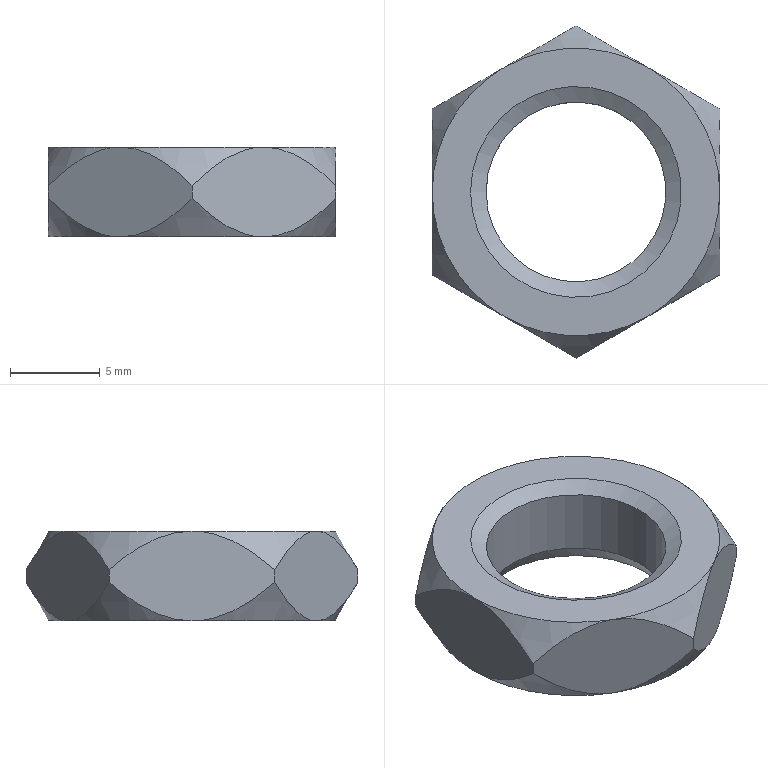Part | NX | features solid 2 | 1 solid | 23 faces | box 16 x 18.475 x 5 mm | volume 674.901 mm3 | cone 14 | plane 8 | cylinder 1 | commonest cylinder face diameters 10 x1
STEP:
#1=CARTESIAN_POINT('',(-5.5,537.,-71.));
#2=VERTEX_POINT('',#1);
#3=CARTESIAN_POINT('',(0.,537.,-71.));
#4=DIRECTION('',(0.,0.,-1.));
#5=DIRECTION('',(-1.,0.,0.));
#6=AXIS2_PLACEMENT_3D('',#3,#4,#5);
#7=CIRCLE('',#6,5.5);
#8=EDGE_CURVE('',#2,#2,#7,.F.);
#9=ORIENTED_EDGE('',*,*,#8,.T.);
#10=EDGE_LOOP('',(#9));
#11=FACE_BOUND('',#10,.T.);
#12=CARTESIAN_POINT('',(-8.,537.,-71.));
#13=VERTEX_POINT('',#12);
#14=CARTESIAN_POINT('',(-4.,530.072,-71.));
#15=VERTEX_POINT('',#14);
#16=CARTESIAN_POINT('',(0.,537.,-71.));
#17=DIRECTION('',(0.,0.,1.));
#18=DIRECTION('',(1.,0.,0.));
#19=AXIS2_PLACEMENT_3D('',#16,#17,#18);
#20=CIRCLE('',#19,8.);
#21=EDGE_CURVE('',#13,#15,#20,.T.);
#22=ORIENTED_EDGE('',*,*,#21,.F.);
#23=CARTESIAN_POINT('',(-4.,543.928,-71.));
#24=VERTEX_POINT('',#23);
#25=CARTESIAN_POINT('',(0.,537.,-71.));
#26=DIRECTION('',(0.,0.,1.));
#27=DIRECTION('',(1.,0.,0.));
#28=AXIS2_PLACEMENT_3D('',#25,#26,#27);
#29=CIRCLE('',#28,8.);
#30=EDGE_CURVE('',#24,#13,#29,.T.);
#31=ORIENTED_EDGE('',*,*,#30,.F.);
#32=CARTESIAN_POINT('',(4.,543.928,-71.));
#33=VERTEX_POINT('',#32);
#34=CARTESIAN_POINT('',(0.,537.,-71.));
#35=DIRECTION('',(0.,0.,1.));
#36=DIRECTION('',(1.,0.,0.));
#37=AXIS2_PLACEMENT_3D('',#34,#35,#36);
#38=CIRCLE('',#37,8.);
#39=EDGE_CURVE('',#33,#24,#38,.T.);
#40=ORIENTED_EDGE('',*,*,#39,.F.);
#41=CARTESIAN_POINT('',(8.,537.,-71.));
#42=VERTEX_POINT('',#41);
#43=CARTESIAN_POINT('',(0.,537.,-71.));
#44=DIRECTION('',(0.,0.,1.));
#45=DIRECTION('',(1.,0.,0.));
#46=AXIS2_PLACEMENT_3D('',#43,#44,#45);
#47=CIRCLE('',#46,8.);
#48=EDGE_CURVE('',#42,#33,#47,.T.);
#49=ORIENTED_EDGE('',*,*,#48,.F.);
#50=CARTESIAN_POINT('',(4.,530.072,-71.));
#51=VERTEX_POINT('',#50);
#52=CARTESIAN_POINT('',(0.,537.,-71.));
#53=DIRECTION('',(0.,0.,1.));
#54=DIRECTION('',(1.,0.,0.));
#55=AXIS2_PLACEMENT_3D('',#52,#53,#54);
#56=CIRCLE('',#55,8.);
#57=EDGE_CURVE('',#51,#42,#56,.T.);
#58=ORIENTED_EDGE('',*,*,#57,.F.);
#59=CARTESIAN_POINT('',(0.,537.,-71.));
#60=DIRECTION('',(0.,0.,1.));
#61=DIRECTION('',(1.,0.,0.));
#62=AXIS2_PLACEMENT_3D('',#59,#60,#61);
#63=CIRCLE('',#62,8.);
#64=EDGE_CURVE('',#15,#51,#63,.T.);
#65=ORIENTED_EDGE('',*,*,#64,.F.);
#66=EDGE_LOOP('',(#22,#31,#40,#49,#58,#65));
#67=FACE_BOUND('',#66,.T.);
#68=CARTESIAN_POINT('',(-16.,537.,-71.));
#69=DIRECTION('',(0.,0.,-1.));
#70=DIRECTION('',(-1.,0.,0.));
#71=AXIS2_PLACEMENT_3D('',#68,#69,#70);
#72=PLANE('',#71);
#73=ADVANCED_FACE('',(#11,#67),#72,.T.);
#74=CARTESIAN_POINT('',(-8.,532.381,-68.144));
#75=VERTEX_POINT('',#74);
#76=CARTESIAN_POINT('',(-4.,530.072,-66.));
#77=VERTEX_POINT('',#76);
#78=CARTESIAN_POINT('',(-8.,532.381,-68.144));
#79=CARTESIAN_POINT('',(-7.431,532.053,-67.575));
#80=CARTESIAN_POINT('',(-6.238,531.364,-66.534));
#81=CARTESIAN_POINT('',(-4.752,530.506,-66.));
#82=CARTESIAN_POINT('',(-4.,530.072,-66.));
#83=B_SPLINE_CURVE_WITH_KNOTS('',3,(#78,#79,#80,#81,#82),.UNSPECIFIED.,.F.,.F.,(4,1,4),(0.000000303,0.002586,0.005171),.UNSPECIFIED.);
#84=EDGE_CURVE('',#75,#77,#83,.T.);
#85=ORIENTED_EDGE('',*,*,#84,.F.);
#86=CARTESIAN_POINT('',(-8.,532.381,-68.856));
#87=VERTEX_POINT('',#86);
#88=CARTESIAN_POINT('',(-8.,532.381,-66.));
#89=DIRECTION('',(0.,0.,-1.));
#90=VECTOR('',#89,1000.);
#91=LINE('',#88,#90);
#92=EDGE_CURVE('',#75,#87,#91,.T.);
#93=ORIENTED_EDGE('',*,*,#92,.T.);
#94=CARTESIAN_POINT('',(-8.,532.381,-68.856));
#95=CARTESIAN_POINT('',(-7.431,532.053,-69.425));
#96=CARTESIAN_POINT('',(-6.238,531.364,-70.466));
#97=CARTESIAN_POINT('',(-4.752,530.506,-71.));
#98=CARTESIAN_POINT('',(-4.,530.072,-71.));
#99=B_SPLINE_CURVE_WITH_KNOTS('',3,(#94,#95,#96,#97,#98),.UNSPECIFIED.,.F.,.F.,(4,1,4),(0.000000303,0.002586,0.005171),.UNSPECIFIED.);
#100=EDGE_CURVE('',#87,#15,#99,.T.);
#101=ORIENTED_EDGE('',*,*,#100,.T.);
#102=CARTESIAN_POINT('',(0.,527.762,-68.856));
#103=VERTEX_POINT('',#102);
#104=CARTESIAN_POINT('',(-4.,530.072,-71.));
#105=CARTESIAN_POINT('',(-2.498,529.205,-71.));
#106=CARTESIAN_POINT('',(-1.14,528.42,-69.996));
#107=CARTESIAN_POINT('',(0.,527.762,-68.856));
#108=B_SPLINE_CURVE_WITH_KNOTS('',3,(#104,#105,#106,#107),.UNSPECIFIED.,.F.,.F.,(4,4),(0.005171,0.01033),.UNSPECIFIED.);
#109=EDGE_CURVE('',#15,#103,#108,.T.);
#110=ORIENTED_EDGE('',*,*,#109,.T.);
#111=CARTESIAN_POINT('',(0.,527.762,-68.144));
#112=VERTEX_POINT('',#111);
#113=CARTESIAN_POINT('',(0.,527.762,-66.));
#114=DIRECTION('',(0.,0.,-1.));
#115=VECTOR('',#114,1000.);
#116=LINE('',#113,#115);
#117=EDGE_CURVE('',#112,#103,#116,.T.);
#118=ORIENTED_EDGE('',*,*,#117,.F.);
#119=CARTESIAN_POINT('',(-4.,530.072,-66.));
#120=CARTESIAN_POINT('',(-2.498,529.205,-66.));
#121=CARTESIAN_POINT('',(-1.14,528.42,-67.004));
#122=CARTESIAN_POINT('',(0.,527.762,-68.144));
#123=B_SPLINE_CURVE_WITH_KNOTS('',3,(#119,#120,#121,#122),.UNSPECIFIED.,.F.,.F.,(4,4),(0.005171,0.01033),.UNSPECIFIED.);
#124=EDGE_CURVE('',#77,#112,#123,.T.);
#125=ORIENTED_EDGE('',*,*,#124,.F.);
#126=EDGE_LOOP('',(#85,#93,#101,#110,#118,#125));
#127=FACE_BOUND('',#126,.T.);
#128=CARTESIAN_POINT('',(0.,527.762,-66.));
#129=DIRECTION('',(-0.5,-0.866,0.));
#130=DIRECTION('',(0.866,-0.5,0.));
#131=AXIS2_PLACEMENT_3D('',#128,#129,#130);
#132=PLANE('',#131);
#133=ADVANCED_FACE('',(#127),#132,.T.);
#134=CARTESIAN_POINT('',(-8.,541.619,-68.144));
#135=VERTEX_POINT('',#134);
#136=CARTESIAN_POINT('',(-8.,537.,-66.));
#137=VERTEX_POINT('',#136);
#138=CARTESIAN_POINT('',(-8.,537.,-66.));
#139=CARTESIAN_POINT('',(-8.,538.745,-66.));
#140=CARTESIAN_POINT('',(-8.,540.316,-67.015));
#141=CARTESIAN_POINT('',(-8.,541.619,-68.144));
#142=B_SPLINE_CURVE_WITH_KNOTS('',3,(#138,#139,#140,#141),.UNSPECIFIED.,.F.,.F.,(4,4),(0.01058,0.01572),.UNSPECIFIED.);
#143=EDGE_CURVE('',#135,#137,#142,.F.);
#144=ORIENTED_EDGE('',*,*,#143,.F.);
#145=CARTESIAN_POINT('',(-8.,541.619,-68.856));
#146=VERTEX_POINT('',#145);
#147=CARTESIAN_POINT('',(-8.,541.619,-66.));
#148=DIRECTION('',(0.,0.,-1.));
#149=VECTOR('',#148,1000.);
#150=LINE('',#147,#149);
#151=EDGE_CURVE('',#135,#146,#150,.T.);
#152=ORIENTED_EDGE('',*,*,#151,.T.);
#153=CARTESIAN_POINT('',(-8.,537.,-71.));
#154=CARTESIAN_POINT('',(-8.,538.745,-71.));
#155=CARTESIAN_POINT('',(-8.,540.316,-69.985));
#156=CARTESIAN_POINT('',(-8.,541.619,-68.856));
#157=B_SPLINE_CURVE_WITH_KNOTS('',3,(#153,#154,#155,#156),.UNSPECIFIED.,.F.,.F.,(4,4),(0.01058,0.01572),.UNSPECIFIED.);
#158=EDGE_CURVE('',#146,#13,#157,.F.);
#159=ORIENTED_EDGE('',*,*,#158,.T.);
#160=CARTESIAN_POINT('',(-8.,532.381,-68.856));
#161=CARTESIAN_POINT('',(-8.,533.681,-69.982));
#162=CARTESIAN_POINT('',(-8.,535.253,-71.));
#163=CARTESIAN_POINT('',(-8.,537.,-71.));
#164=B_SPLINE_CURVE_WITH_KNOTS('',3,(#160,#161,#162,#163),.UNSPECIFIED.,.F.,.F.,(4,4),(0.005438,0.01058),.UNSPECIFIED.);
#165=EDGE_CURVE('',#13,#87,#164,.F.);
#166=ORIENTED_EDGE('',*,*,#165,.T.);
#167=ORIENTED_EDGE('',*,*,#92,.F.);
#168=CARTESIAN_POINT('',(-8.,532.381,-68.144));
#169=CARTESIAN_POINT('',(-8.,533.681,-67.018));
#170=CARTESIAN_POINT('',(-8.,535.253,-66.));
#171=CARTESIAN_POINT('',(-8.,537.,-66.));
#172=B_SPLINE_CURVE_WITH_KNOTS('',3,(#168,#169,#170,#171),.UNSPECIFIED.,.F.,.F.,(4,4),(0.005438,0.01058),.UNSPECIFIED.);
#173=EDGE_CURVE('',#137,#75,#172,.F.);
#174=ORIENTED_EDGE('',*,*,#173,.F.);
#175=EDGE_LOOP('',(#144,#152,#159,#166,#167,#174));
#176=FACE_BOUND('',#175,.T.);
#177=CARTESIAN_POINT('',(-8.,532.381,-66.));
#178=DIRECTION('',(-1.,0.,0.));
#179=DIRECTION('',(0.,0.,1.));
#180=AXIS2_PLACEMENT_3D('',#177,#178,#179);
#181=PLANE('',#180);
#182=ADVANCED_FACE('',(#176),#181,.T.);
#183=CARTESIAN_POINT('',(0.,546.238,-68.144));
#184=VERTEX_POINT('',#183);
#185=CARTESIAN_POINT('',(-4.,543.928,-66.));
#186=VERTEX_POINT('',#185);
#187=CARTESIAN_POINT('',(0.,546.238,-68.144));
#188=CARTESIAN_POINT('',(-0.5691,545.909,-67.575));
#189=CARTESIAN_POINT('',(-1.762,545.221,-66.534));
#190=CARTESIAN_POINT('',(-3.248,544.362,-66.));
#191=CARTESIAN_POINT('',(-4.,543.928,-66.));
#192=B_SPLINE_CURVE_WITH_KNOTS('',3,(#187,#188,#189,#190,#191),.UNSPECIFIED.,.F.,.F.,(4,1,4),(0.000000303,0.002586,0.005171),.UNSPECIFIED.);
#193=EDGE_CURVE('',#184,#186,#192,.T.);
#194=ORIENTED_EDGE('',*,*,#193,.F.);
#195=CARTESIAN_POINT('',(0.,546.238,-68.856));
#196=VERTEX_POINT('',#195);
#197=CARTESIAN_POINT('',(0.,546.238,-66.));
#198=DIRECTION('',(0.,0.,-1.));
#199=VECTOR('',#198,1000.);
#200=LINE('',#197,#199);
#201=EDGE_CURVE('',#184,#196,#200,.T.);
#202=ORIENTED_EDGE('',*,*,#201,.T.);
#203=CARTESIAN_POINT('',(0.,546.238,-68.856));
#204=CARTESIAN_POINT('',(-0.5691,545.909,-69.425));
#205=CARTESIAN_POINT('',(-1.762,545.221,-70.466));
#206=CARTESIAN_POINT('',(-3.248,544.362,-71.));
#207=CARTESIAN_POINT('',(-4.,543.928,-71.));
#208=B_SPLINE_CURVE_WITH_KNOTS('',3,(#203,#204,#205,#206,#207),.UNSPECIFIED.,.F.,.F.,(4,1,4),(0.000000303,0.002586,0.005171),.UNSPECIFIED.);
#209=EDGE_CURVE('',#196,#24,#208,.T.);
#210=ORIENTED_EDGE('',*,*,#209,.T.);
#211=CARTESIAN_POINT('',(-4.,543.928,-71.));
#212=CARTESIAN_POINT('',(-5.502,543.061,-71.));
#213=CARTESIAN_POINT('',(-6.86,542.277,-69.996));
#214=CARTESIAN_POINT('',(-8.,541.619,-68.856));
#215=B_SPLINE_CURVE_WITH_KNOTS('',3,(#211,#212,#213,#214),.UNSPECIFIED.,.F.,.F.,(4,4),(0.005171,0.01033),.UNSPECIFIED.);
#216=EDGE_CURVE('',#24,#146,#215,.T.);
#217=ORIENTED_EDGE('',*,*,#216,.T.);
#218=ORIENTED_EDGE('',*,*,#151,.F.);
#219=CARTESIAN_POINT('',(-4.,543.928,-66.));
#220=CARTESIAN_POINT('',(-5.502,543.061,-66.));
#221=CARTESIAN_POINT('',(-6.86,542.277,-67.004));
#222=CARTESIAN_POINT('',(-8.,541.619,-68.144));
#223=B_SPLINE_CURVE_WITH_KNOTS('',3,(#219,#220,#221,#222),.UNSPECIFIED.,.F.,.F.,(4,4),(0.005171,0.01033),.UNSPECIFIED.);
#224=EDGE_CURVE('',#186,#135,#223,.T.);
#225=ORIENTED_EDGE('',*,*,#224,.F.);
#226=EDGE_LOOP('',(#194,#202,#210,#217,#218,#225));
#227=FACE_BOUND('',#226,.T.);
#228=CARTESIAN_POINT('',(-8.,541.619,-66.));
#229=DIRECTION('',(-0.5,0.866,0.));
#230=DIRECTION('',(-0.866,-0.5,0.));
#231=AXIS2_PLACEMENT_3D('',#228,#229,#230);
#232=PLANE('',#231);
#233=ADVANCED_FACE('',(#227),#232,.T.);
#234=CARTESIAN_POINT('',(8.,541.619,-68.144));
#235=VERTEX_POINT('',#234);
#236=CARTESIAN_POINT('',(4.,543.928,-66.));
#237=VERTEX_POINT('',#236);
#238=CARTESIAN_POINT('',(8.,541.619,-68.144));
#239=CARTESIAN_POINT('',(7.431,541.947,-67.575));
#240=CARTESIAN_POINT('',(6.238,542.636,-66.534));
#241=CARTESIAN_POINT('',(4.752,543.494,-66.));
#242=CARTESIAN_POINT('',(4.,543.928,-66.));
#243=B_SPLINE_CURVE_WITH_KNOTS('',3,(#238,#239,#240,#241,#242),.UNSPECIFIED.,.F.,.F.,(4,1,4),(0.000000303,0.002586,0.005171),.UNSPECIFIED.);
#244=EDGE_CURVE('',#235,#237,#243,.T.);
#245=ORIENTED_EDGE('',*,*,#244,.F.);
#246=CARTESIAN_POINT('',(8.,541.619,-68.856));
#247=VERTEX_POINT('',#246);
#248=CARTESIAN_POINT('',(8.,541.619,-66.));
#249=DIRECTION('',(0.,0.,-1.));
#250=VECTOR('',#249,1000.);
#251=LINE('',#248,#250);
#252=EDGE_CURVE('',#235,#247,#251,.T.);
#253=ORIENTED_EDGE('',*,*,#252,.T.);
#254=CARTESIAN_POINT('',(8.,541.619,-68.856));
#255=CARTESIAN_POINT('',(7.431,541.947,-69.425));
#256=CARTESIAN_POINT('',(6.238,542.636,-70.466));
#257=CARTESIAN_POINT('',(4.752,543.494,-71.));
#258=CARTESIAN_POINT('',(4.,543.928,-71.));
#259=B_SPLINE_CURVE_WITH_KNOTS('',3,(#254,#255,#256,#257,#258),.UNSPECIFIED.,.F.,.F.,(4,1,4),(0.000000303,0.002586,0.005171),.UNSPECIFIED.);
#260=EDGE_CURVE('',#247,#33,#259,.T.);
#261=ORIENTED_EDGE('',*,*,#260,.T.);
#262=CARTESIAN_POINT('',(4.,543.928,-71.));
#263=CARTESIAN_POINT('',(2.498,544.795,-71.));
#264=CARTESIAN_POINT('',(1.14,545.58,-69.996));
#265=CARTESIAN_POINT('',(0.,546.238,-68.856));
#266=B_SPLINE_CURVE_WITH_KNOTS('',3,(#262,#263,#264,#265),.UNSPECIFIED.,.F.,.F.,(4,4),(0.005171,0.01033),.UNSPECIFIED.);
#267=EDGE_CURVE('',#33,#196,#266,.T.);
#268=ORIENTED_EDGE('',*,*,#267,.T.);
#269=ORIENTED_EDGE('',*,*,#201,.F.);
#270=CARTESIAN_POINT('',(4.,543.928,-66.));
#271=CARTESIAN_POINT('',(2.498,544.795,-66.));
#272=CARTESIAN_POINT('',(1.14,545.58,-67.004));
#273=CARTESIAN_POINT('',(0.,546.238,-68.144));
#274=B_SPLINE_CURVE_WITH_KNOTS('',3,(#270,#271,#272,#273),.UNSPECIFIED.,.F.,.F.,(4,4),(0.005171,0.01033),.UNSPECIFIED.);
#275=EDGE_CURVE('',#237,#184,#274,.T.);
#276=ORIENTED_EDGE('',*,*,#275,.F.);
#277=EDGE_LOOP('',(#245,#253,#261,#268,#269,#276));
#278=FACE_BOUND('',#277,.T.);
#279=CARTESIAN_POINT('',(0.,546.238,-66.));
#280=DIRECTION('',(0.5,0.866,0.));
#281=DIRECTION('',(-0.866,0.5,0.));
#282=AXIS2_PLACEMENT_3D('',#279,#280,#281);
#283=PLANE('',#282);
#284=ADVANCED_FACE('',(#278),#283,.T.);
#285=CARTESIAN_POINT('',(8.,532.381,-68.144));
#286=VERTEX_POINT('',#285);
#287=CARTESIAN_POINT('',(8.,537.,-66.));
#288=VERTEX_POINT('',#287);
#289=CARTESIAN_POINT('',(8.,532.381,-68.144));
#290=CARTESIAN_POINT('',(8.,533.681,-67.018));
#291=CARTESIAN_POINT('',(8.,535.253,-66.));
#292=CARTESIAN_POINT('',(8.,537.,-66.));
#293=B_SPLINE_CURVE_WITH_KNOTS('',3,(#289,#290,#291,#292),.UNSPECIFIED.,.F.,.F.,(4,4),(0.005438,0.01058),.UNSPECIFIED.);
#294=EDGE_CURVE('',#286,#288,#293,.T.);
#295=ORIENTED_EDGE('',*,*,#294,.F.);
#296=CARTESIAN_POINT('',(8.,532.381,-68.856));
#297=VERTEX_POINT('',#296);
#298=CARTESIAN_POINT('',(8.,532.381,-66.));
#299=DIRECTION('',(0.,0.,-1.));
#300=VECTOR('',#299,1000.);
#301=LINE('',#298,#300);
#302=EDGE_CURVE('',#286,#297,#301,.T.);
#303=ORIENTED_EDGE('',*,*,#302,.T.);
#304=CARTESIAN_POINT('',(8.,532.381,-68.856));
#305=CARTESIAN_POINT('',(8.,533.681,-69.982));
#306=CARTESIAN_POINT('',(8.,535.253,-71.));
#307=CARTESIAN_POINT('',(8.,537.,-71.));
#308=B_SPLINE_CURVE_WITH_KNOTS('',3,(#304,#305,#306,#307),.UNSPECIFIED.,.F.,.F.,(4,4),(0.005438,0.01058),.UNSPECIFIED.);
#309=EDGE_CURVE('',#297,#42,#308,.T.);
#310=ORIENTED_EDGE('',*,*,#309,.T.);
#311=CARTESIAN_POINT('',(8.,537.,-71.));
#312=CARTESIAN_POINT('',(8.,538.745,-71.));
#313=CARTESIAN_POINT('',(8.,540.316,-69.985));
#314=CARTESIAN_POINT('',(8.,541.619,-68.856));
#315=B_SPLINE_CURVE_WITH_KNOTS('',3,(#311,#312,#313,#314),.UNSPECIFIED.,.F.,.F.,(4,4),(0.01058,0.01572),.UNSPECIFIED.);
#316=EDGE_CURVE('',#42,#247,#315,.T.);
#317=ORIENTED_EDGE('',*,*,#316,.T.);
#318=ORIENTED_EDGE('',*,*,#252,.F.);
#319=CARTESIAN_POINT('',(8.,537.,-66.));
#320=CARTESIAN_POINT('',(8.,538.745,-66.));
#321=CARTESIAN_POINT('',(8.,540.316,-67.015));
#322=CARTESIAN_POINT('',(8.,541.619,-68.144));
#323=B_SPLINE_CURVE_WITH_KNOTS('',3,(#319,#320,#321,#322),.UNSPECIFIED.,.F.,.F.,(4,4),(0.01058,0.01572),.UNSPECIFIED.);
#324=EDGE_CURVE('',#288,#235,#323,.T.);
#325=ORIENTED_EDGE('',*,*,#324,.F.);
#326=EDGE_LOOP('',(#295,#303,#310,#317,#318,#325));
#327=FACE_BOUND('',#326,.T.);
#328=CARTESIAN_POINT('',(8.,541.619,-66.));
#329=DIRECTION('',(1.,0.,0.));
#330=DIRECTION('',(0.,0.,-1.));
#331=AXIS2_PLACEMENT_3D('',#328,#329,#330);
#332=PLANE('',#331);
#333=ADVANCED_FACE('',(#327),#332,.T.);
#334=CARTESIAN_POINT('',(4.,530.072,-66.));
#335=VERTEX_POINT('',#334);
#336=CARTESIAN_POINT('',(0.,527.762,-68.144));
#337=CARTESIAN_POINT('',(0.5691,528.091,-67.575));
#338=CARTESIAN_POINT('',(1.762,528.779,-66.534));
#339=CARTESIAN_POINT('',(3.248,529.638,-66.));
#340=CARTESIAN_POINT('',(4.,530.072,-66.));
#341=B_SPLINE_CURVE_WITH_KNOTS('',3,(#336,#337,#338,#339,#340),.UNSPECIFIED.,.F.,.F.,(4,1,4),(0.000000303,0.002586,0.005171),.UNSPECIFIED.);
#342=EDGE_CURVE('',#112,#335,#341,.T.);
#343=ORIENTED_EDGE('',*,*,#342,.F.);
#344=ORIENTED_EDGE('',*,*,#117,.T.);
#345=CARTESIAN_POINT('',(0.,527.762,-68.856));
#346=CARTESIAN_POINT('',(0.5691,528.091,-69.425));
#347=CARTESIAN_POINT('',(1.762,528.779,-70.466));
#348=CARTESIAN_POINT('',(3.248,529.638,-71.));
#349=CARTESIAN_POINT('',(4.,530.072,-71.));
#350=B_SPLINE_CURVE_WITH_KNOTS('',3,(#345,#346,#347,#348,#349),.UNSPECIFIED.,.F.,.F.,(4,1,4),(0.000000303,0.002586,0.005171),.UNSPECIFIED.);
#351=EDGE_CURVE('',#103,#51,#350,.T.);
#352=ORIENTED_EDGE('',*,*,#351,.T.);
#353=CARTESIAN_POINT('',(4.,530.072,-71.));
#354=CARTESIAN_POINT('',(5.502,530.939,-71.));
#355=CARTESIAN_POINT('',(6.86,531.723,-69.996));
#356=CARTESIAN_POINT('',(8.,532.381,-68.856));
#357=B_SPLINE_CURVE_WITH_KNOTS('',3,(#353,#354,#355,#356),.UNSPECIFIED.,.F.,.F.,(4,4),(0.005171,0.01033),.UNSPECIFIED.);
#358=EDGE_CURVE('',#51,#297,#357,.T.);
#359=ORIENTED_EDGE('',*,*,#358,.T.);
#360=ORIENTED_EDGE('',*,*,#302,.F.);
#361=CARTESIAN_POINT('',(4.,530.072,-66.));
#362=CARTESIAN_POINT('',(5.502,530.939,-66.));
#363=CARTESIAN_POINT('',(6.86,531.723,-67.004));
#364=CARTESIAN_POINT('',(8.,532.381,-68.144));
#365=B_SPLINE_CURVE_WITH_KNOTS('',3,(#361,#362,#363,#364),.UNSPECIFIED.,.F.,.F.,(4,4),(0.005171,0.01033),.UNSPECIFIED.);
#366=EDGE_CURVE('',#335,#286,#365,.T.);
#367=ORIENTED_EDGE('',*,*,#366,.F.);
#368=EDGE_LOOP('',(#343,#344,#352,#359,#360,#367));
#369=FACE_BOUND('',#368,.T.);
#370=CARTESIAN_POINT('',(8.,532.381,-66.));
#371=DIRECTION('',(0.5,-0.866,0.));
#372=DIRECTION('',(0.866,0.5,0.));
#373=AXIS2_PLACEMENT_3D('',#370,#371,#372);
#374=PLANE('',#373);
#375=ADVANCED_FACE('',(#369),#374,.T.);
#376=CARTESIAN_POINT('',(-5.866,537.,-66.));
#377=VERTEX_POINT('',#376);
#378=CARTESIAN_POINT('',(0.,537.,-66.));
#379=DIRECTION('',(0.,0.,-1.));
#380=DIRECTION('',(-1.,0.,0.));
#381=AXIS2_PLACEMENT_3D('',#378,#379,#380);
#382=CIRCLE('',#381,5.866);
#383=EDGE_CURVE('',#377,#377,#382,.T.);
#384=ORIENTED_EDGE('',*,*,#383,.T.);
#385=EDGE_LOOP('',(#384));
#386=FACE_BOUND('',#385,.T.);
#387=CARTESIAN_POINT('',(0.,537.,-66.));
#388=DIRECTION('',(0.,0.,-1.));
#389=DIRECTION('',(-1.,0.,0.));
#390=AXIS2_PLACEMENT_3D('',#387,#388,#389);
#391=CIRCLE('',#390,8.);
#392=EDGE_CURVE('',#186,#137,#391,.F.);
#393=ORIENTED_EDGE('',*,*,#392,.T.);
#394=CARTESIAN_POINT('',(0.,537.,-66.));
#395=DIRECTION('',(0.,0.,-1.));
#396=DIRECTION('',(-1.,0.,0.));
#397=AXIS2_PLACEMENT_3D('',#394,#395,#396);
#398=CIRCLE('',#397,8.);
#399=EDGE_CURVE('',#137,#77,#398,.F.);
#400=ORIENTED_EDGE('',*,*,#399,.T.);
#401=CARTESIAN_POINT('',(0.,537.,-66.));
#402=DIRECTION('',(0.,0.,-1.));
#403=DIRECTION('',(-1.,0.,0.));
#404=AXIS2_PLACEMENT_3D('',#401,#402,#403);
#405=CIRCLE('',#404,8.);
#406=EDGE_CURVE('',#77,#335,#405,.F.);
#407=ORIENTED_EDGE('',*,*,#406,.T.);
#408=CARTESIAN_POINT('',(0.,537.,-66.));
#409=DIRECTION('',(0.,0.,-1.));
#410=DIRECTION('',(-1.,0.,0.));
#411=AXIS2_PLACEMENT_3D('',#408,#409,#410);
#412=CIRCLE('',#411,8.);
#413=EDGE_CURVE('',#335,#288,#412,.F.);
#414=ORIENTED_EDGE('',*,*,#413,.T.);
#415=CARTESIAN_POINT('',(0.,537.,-66.));
#416=DIRECTION('',(0.,0.,1.));
#417=DIRECTION('',(1.,0.,0.));
#418=AXIS2_PLACEMENT_3D('',#415,#416,#417);
#419=CIRCLE('',#418,8.);
#420=EDGE_CURVE('',#288,#237,#419,.T.);
#421=ORIENTED_EDGE('',*,*,#420,.T.);
#422=CARTESIAN_POINT('',(0.,537.,-66.));
#423=DIRECTION('',(0.,0.,-1.));
#424=DIRECTION('',(-1.,0.,0.));
#425=AXIS2_PLACEMENT_3D('',#422,#423,#424);
#426=CIRCLE('',#425,8.);
#427=EDGE_CURVE('',#237,#186,#426,.F.);
#428=ORIENTED_EDGE('',*,*,#427,.T.);
#429=EDGE_LOOP('',(#393,#400,#407,#414,#421,#428));
#430=FACE_BOUND('',#429,.T.);
#431=CARTESIAN_POINT('',(-16.,537.,-66.));
#432=DIRECTION('',(0.,0.,-1.));
#433=DIRECTION('',(-1.,0.,0.));
#434=AXIS2_PLACEMENT_3D('',#431,#432,#433);
#435=PLANE('',#434);
#436=ADVANCED_FACE('',(#386,#430),#435,.F.);
#437=CARTESIAN_POINT('',(-5.,537.,-70.134));
#438=VERTEX_POINT('',#437);
#439=CARTESIAN_POINT('',(0.,537.,-70.134));
#440=DIRECTION('',(0.,0.,-1.));
#441=DIRECTION('',(-1.,0.,0.));
#442=AXIS2_PLACEMENT_3D('',#439,#440,#441);
#443=CIRCLE('',#442,5.);
#444=EDGE_CURVE('',#438,#438,#443,.T.);
#445=ORIENTED_EDGE('',*,*,#444,.T.);
#446=EDGE_LOOP('',(#445));
#447=FACE_BOUND('',#446,.T.);
#448=CARTESIAN_POINT('',(-5.,537.,-66.5));
#449=VERTEX_POINT('',#448);
#450=CARTESIAN_POINT('',(0.,537.,-66.5));
#451=DIRECTION('',(0.,0.,-1.));
#452=DIRECTION('',(-1.,0.,0.));
#453=AXIS2_PLACEMENT_3D('',#450,#451,#452);
#454=CIRCLE('',#453,5.);
#455=EDGE_CURVE('',#449,#449,#454,.F.);
#456=ORIENTED_EDGE('',*,*,#455,.T.);
#457=EDGE_LOOP('',(#456));
#458=FACE_BOUND('',#457,.T.);
#459=CARTESIAN_POINT('',(0.,537.,-66.));
#460=DIRECTION('',(0.,0.,-1.));
#461=DIRECTION('',(-1.,0.,0.));
#462=AXIS2_PLACEMENT_3D('',#459,#460,#461);
#463=CYLINDRICAL_SURFACE('',#462,5.);
#464=ADVANCED_FACE('',(#447,#458),#463,.F.);
#465=ORIENTED_EDGE('',*,*,#383,.F.);
#466=EDGE_LOOP('',(#465));
#467=FACE_BOUND('',#466,.T.);
#468=ORIENTED_EDGE('',*,*,#455,.F.);
#469=EDGE_LOOP('',(#468));
#470=FACE_BOUND('',#469,.T.);
#471=CARTESIAN_POINT('',(0.,537.,-66.5));
#472=DIRECTION('',(0.,0.,1.));
#473=DIRECTION('',(1.,0.,0.));
#474=AXIS2_PLACEMENT_3D('',#471,#472,#473);
#475=CONICAL_SURFACE('',#474,5.,1.047);
#476=ADVANCED_FACE('',(#467,#470),#475,.F.);
#477=ORIENTED_EDGE('',*,*,#444,.F.);
#478=EDGE_LOOP('',(#477));
#479=FACE_BOUND('',#478,.T.);
#480=ORIENTED_EDGE('',*,*,#8,.F.);
#481=EDGE_LOOP('',(#480));
#482=FACE_BOUND('',#481,.T.);
#483=CARTESIAN_POINT('',(0.,537.,-71.));
#484=DIRECTION('',(0.,0.,-1.));
#485=DIRECTION('',(-1.,0.,0.));
#486=AXIS2_PLACEMENT_3D('',#483,#484,#485);
#487=CONICAL_SURFACE('',#486,5.5,0.5236);
#488=ADVANCED_FACE('',(#479,#482),#487,.F.);
#489=ORIENTED_EDGE('',*,*,#358,.F.);
#490=ORIENTED_EDGE('',*,*,#57,.T.);
#491=ORIENTED_EDGE('',*,*,#309,.F.);
#492=EDGE_LOOP('',(#489,#490,#491));
#493=FACE_BOUND('',#492,.T.);
#494=CARTESIAN_POINT('',(0.,537.,-71.));
#495=DIRECTION('',(0.,0.,1.));
#496=DIRECTION('',(-1.,0.,0.));
#497=AXIS2_PLACEMENT_3D('',#494,#495,#496);
#498=CONICAL_SURFACE('',#497,8.,0.5236);
#499=ADVANCED_FACE('',(#493),#498,.T.);
#500=ORIENTED_EDGE('',*,*,#64,.T.);
#501=ORIENTED_EDGE('',*,*,#351,.F.);
#502=ORIENTED_EDGE('',*,*,#109,.F.);
#503=EDGE_LOOP('',(#500,#501,#502));
#504=FACE_BOUND('',#503,.T.);
#505=CARTESIAN_POINT('',(0.,537.,-71.));
#506=DIRECTION('',(0.,0.,1.));
#507=DIRECTION('',(-1.,0.,0.));
#508=AXIS2_PLACEMENT_3D('',#505,#506,#507);
#509=CONICAL_SURFACE('',#508,8.,0.5236);
#510=ADVANCED_FACE('',(#504),#509,.T.);
#511=ORIENTED_EDGE('',*,*,#316,.F.);
#512=ORIENTED_EDGE('',*,*,#48,.T.);
#513=ORIENTED_EDGE('',*,*,#260,.F.);
#514=EDGE_LOOP('',(#511,#512,#513));
#515=FACE_BOUND('',#514,.T.);
#516=CARTESIAN_POINT('',(0.,537.,-71.));
#517=DIRECTION('',(0.,0.,1.));
#518=DIRECTION('',(-1.,0.,0.));
#519=AXIS2_PLACEMENT_3D('',#516,#517,#518);
#520=CONICAL_SURFACE('',#519,8.,0.5236);
#521=ADVANCED_FACE('',(#515),#520,.T.);
#522=ORIENTED_EDGE('',*,*,#267,.F.);
#523=ORIENTED_EDGE('',*,*,#39,.T.);
#524=ORIENTED_EDGE('',*,*,#209,.F.);
#525=EDGE_LOOP('',(#522,#523,#524));
#526=FACE_BOUND('',#525,.T.);
#527=CARTESIAN_POINT('',(0.,537.,-71.));
#528=DIRECTION('',(0.,0.,1.));
#529=DIRECTION('',(-1.,0.,0.));
#530=AXIS2_PLACEMENT_3D('',#527,#528,#529);
#531=CONICAL_SURFACE('',#530,8.,0.5236);
#532=ADVANCED_FACE('',(#526),#531,.T.);
#533=ORIENTED_EDGE('',*,*,#30,.T.);
#534=ORIENTED_EDGE('',*,*,#158,.F.);
#535=ORIENTED_EDGE('',*,*,#216,.F.);
#536=EDGE_LOOP('',(#533,#534,#535));
#537=FACE_BOUND('',#536,.T.);
#538=CARTESIAN_POINT('',(0.,537.,-71.));
#539=DIRECTION('',(0.,0.,1.));
#540=DIRECTION('',(-1.,0.,0.));
#541=AXIS2_PLACEMENT_3D('',#538,#539,#540);
#542=CONICAL_SURFACE('',#541,8.,0.5236);
#543=ADVANCED_FACE('',(#537),#542,.T.);
#544=ORIENTED_EDGE('',*,*,#21,.T.);
#545=ORIENTED_EDGE('',*,*,#100,.F.);
#546=ORIENTED_EDGE('',*,*,#165,.F.);
#547=EDGE_LOOP('',(#544,#545,#546));
#548=FACE_BOUND('',#547,.T.);
#549=CARTESIAN_POINT('',(0.,537.,-71.));
#550=DIRECTION('',(0.,0.,1.));
#551=DIRECTION('',(-1.,0.,0.));
#552=AXIS2_PLACEMENT_3D('',#549,#550,#551);
#553=CONICAL_SURFACE('',#552,8.,0.5236);
#554=ADVANCED_FACE('',(#548),#553,.T.);
#555=ORIENTED_EDGE('',*,*,#224,.T.);
#556=ORIENTED_EDGE('',*,*,#143,.T.);
#557=ORIENTED_EDGE('',*,*,#392,.F.);
#558=EDGE_LOOP('',(#555,#556,#557));
#559=FACE_BOUND('',#558,.T.);
#560=CARTESIAN_POINT('',(0.,537.,-66.));
#561=DIRECTION('',(0.,0.,-1.));
#562=DIRECTION('',(-1.,0.,0.));
#563=AXIS2_PLACEMENT_3D('',#560,#561,#562);
#564=CONICAL_SURFACE('',#563,8.,0.5236);
#565=ADVANCED_FACE('',(#559),#564,.T.);
#566=ORIENTED_EDGE('',*,*,#193,.T.);
#567=ORIENTED_EDGE('',*,*,#427,.F.);
#568=ORIENTED_EDGE('',*,*,#275,.T.);
#569=EDGE_LOOP('',(#566,#567,#568));
#570=FACE_BOUND('',#569,.T.);
#571=CARTESIAN_POINT('',(0.,537.,-66.));
#572=DIRECTION('',(0.,0.,-1.));
#573=DIRECTION('',(-1.,0.,0.));
#574=AXIS2_PLACEMENT_3D('',#571,#572,#573);
#575=CONICAL_SURFACE('',#574,8.,0.5236);
#576=ADVANCED_FACE('',(#570),#575,.T.);
#577=ORIENTED_EDGE('',*,*,#244,.T.);
#578=ORIENTED_EDGE('',*,*,#420,.F.);
#579=ORIENTED_EDGE('',*,*,#324,.T.);
#580=EDGE_LOOP('',(#577,#578,#579));
#581=FACE_BOUND('',#580,.T.);
#582=CARTESIAN_POINT('',(0.,537.,-66.));
#583=DIRECTION('',(0.,0.,-1.));
#584=DIRECTION('',(-1.,0.,0.));
#585=AXIS2_PLACEMENT_3D('',#582,#583,#584);
#586=CONICAL_SURFACE('',#585,8.,0.5236);
#587=ADVANCED_FACE('',(#581),#586,.T.);
#588=ORIENTED_EDGE('',*,*,#294,.T.);
#589=ORIENTED_EDGE('',*,*,#413,.F.);
#590=ORIENTED_EDGE('',*,*,#366,.T.);
#591=EDGE_LOOP('',(#588,#589,#590));
#592=FACE_BOUND('',#591,.T.);
#593=CARTESIAN_POINT('',(0.,537.,-66.));
#594=DIRECTION('',(0.,0.,-1.));
#595=DIRECTION('',(-1.,0.,0.));
#596=AXIS2_PLACEMENT_3D('',#593,#594,#595);
#597=CONICAL_SURFACE('',#596,8.,0.5236);
#598=ADVANCED_FACE('',(#592),#597,.T.);
#599=ORIENTED_EDGE('',*,*,#124,.T.);
#600=ORIENTED_EDGE('',*,*,#342,.T.);
#601=ORIENTED_EDGE('',*,*,#406,.F.);
#602=EDGE_LOOP('',(#599,#600,#601));
#603=FACE_BOUND('',#602,.T.);
#604=CARTESIAN_POINT('',(0.,537.,-66.));
#605=DIRECTION('',(0.,0.,-1.));
#606=DIRECTION('',(-1.,0.,0.));
#607=AXIS2_PLACEMENT_3D('',#604,#605,#606);
#608=CONICAL_SURFACE('',#607,8.,0.5236);
#609=ADVANCED_FACE('',(#603),#608,.T.);
#610=ORIENTED_EDGE('',*,*,#173,.T.);
#611=ORIENTED_EDGE('',*,*,#84,.T.);
#612=ORIENTED_EDGE('',*,*,#399,.F.);
#613=EDGE_LOOP('',(#610,#611,#612));
#614=FACE_BOUND('',#613,.T.);
#615=CARTESIAN_POINT('',(0.,537.,-66.));
#616=DIRECTION('',(0.,0.,-1.));
#617=DIRECTION('',(-1.,0.,0.));
#618=AXIS2_PLACEMENT_3D('',#615,#616,#617);
#619=CONICAL_SURFACE('',#618,8.,0.5236);
#620=ADVANCED_FACE('',(#614),#619,.T.);
#621=CLOSED_SHELL('',(#73,#133,#182,#233,#284,#333,#375,#436,#464,#476,#488,#499,#510,#521,#532,#543,#554,#565,#576,#587,#598,#609,#620));
#622=MANIFOLD_SOLID_BREP('',#621);
#623=(LENGTH_UNIT()NAMED_UNIT(*)SI_UNIT(.MILLI.,.METRE.));
#624=UNCERTAINTY_MEASURE_WITH_UNIT(LENGTH_MEASURE(0.0508),#623,'','');
#625=(NAMED_UNIT(*)PLANE_ANGLE_UNIT()SI_UNIT($,.RADIAN.));
#626=(NAMED_UNIT(*)SI_UNIT($,.STERADIAN.)SOLID_ANGLE_UNIT());
#627=(GEOMETRIC_REPRESENTATION_CONTEXT(3)GLOBAL_UNCERTAINTY_ASSIGNED_CONTEXT((#624))GLOBAL_UNIT_ASSIGNED_CONTEXT((#623,#625,#626))REPRESENTATION_CONTEXT('',''));
#628=ADVANCED_BREP_SHAPE_REPRESENTATION('',(#622),#627);